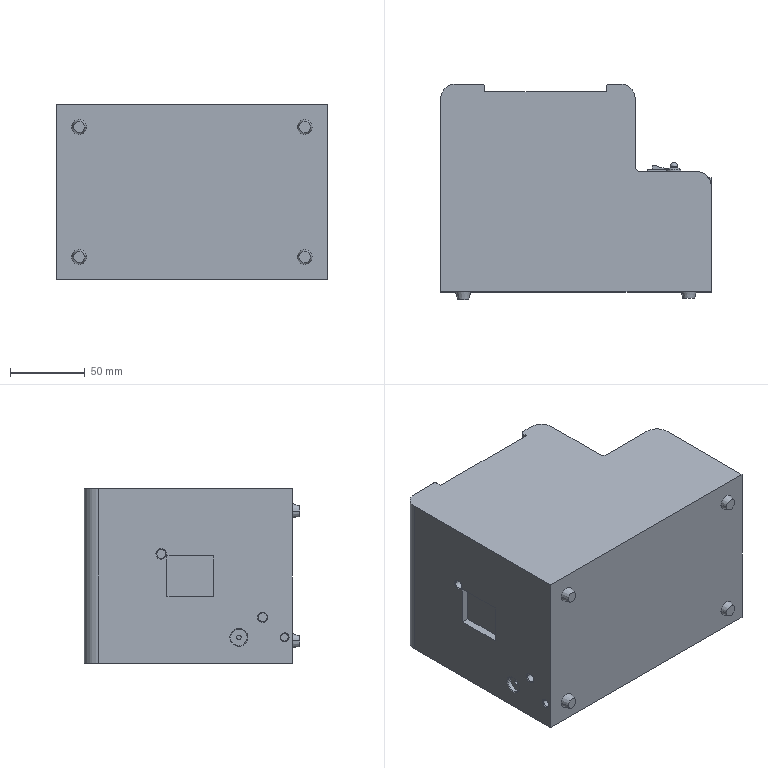Part | STEP file | ASND-0110-SDS_3 | 1 solid | 510 faces | box 181.1 x 144.1 x 117 mm | volume 1395902 mm3 | plane 350 | spline 98 | cylinder 39 | torus 12 | cone 10 | sphere 1 | commonest cylinder face diameters 3 x10 5 x4 6 x4 10 x4 19.2 x4 2 x3